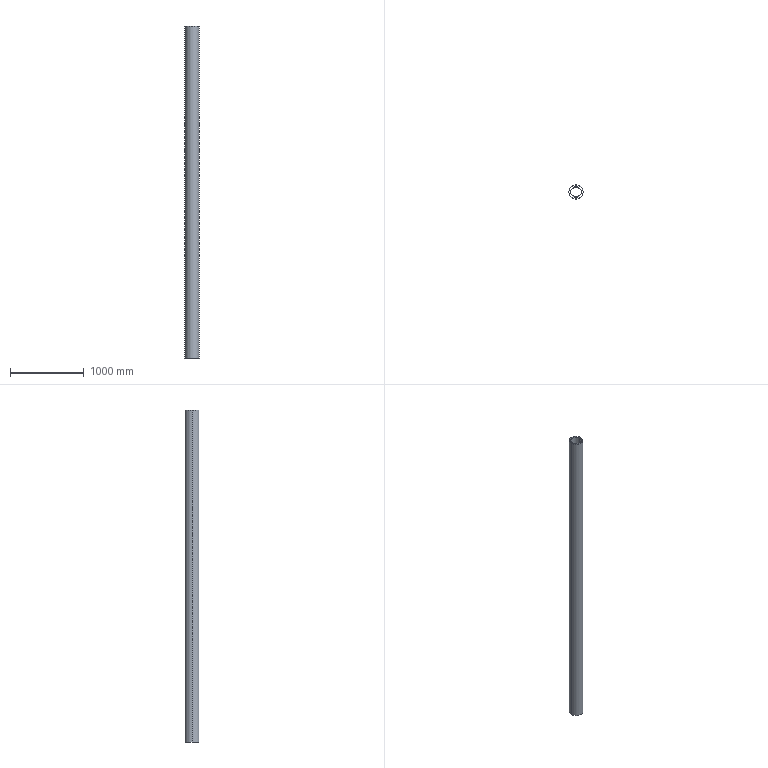Part | SolidWorks | features Extrusion 1, ICE 1 | 2 solids | 12 faces | box 190 x 190 x 4500 mm | volume 116967 mm3 | cylinder 8 | plane 4 | commonest cylinder face diameters 140.95 x2 141 x2 189.95 x2 190 x2
STEP:
#1=CARTESIAN_POINT('',(-94.975,0.,4500.));
#2=VERTEX_POINT('',#1);
#3=CARTESIAN_POINT('',(94.975,0.,4500.));
#4=VERTEX_POINT('',#3);
#5=CARTESIAN_POINT('',(0.,0.,4500.));
#6=DIRECTION('',(0.,0.,1.));
#7=DIRECTION('',(1.,0.,0.));
#8=AXIS2_PLACEMENT_3D('',#5,#6,#7);
#9=CIRCLE('',#8,94.975);
#10=EDGE_CURVE('',#2,#4,#9,.T.);
#11=ORIENTED_EDGE('',*,*,#10,.T.);
#12=CARTESIAN_POINT('',(94.975,0.,0.));
#13=VERTEX_POINT('',#12);
#14=CARTESIAN_POINT('',(94.975,0.,4500.));
#15=DIRECTION('',(0.,0.,-1.));
#16=VECTOR('',#15,1000.);
#17=LINE('',#14,#16);
#18=EDGE_CURVE('',#4,#13,#17,.T.);
#19=ORIENTED_EDGE('',*,*,#18,.T.);
#20=CARTESIAN_POINT('',(-94.975,0.,0.));
#21=VERTEX_POINT('',#20);
#22=CARTESIAN_POINT('',(0.,0.,0.));
#23=DIRECTION('',(0.,0.,1.));
#24=DIRECTION('',(1.,0.,0.));
#25=AXIS2_PLACEMENT_3D('',#22,#23,#24);
#26=CIRCLE('',#25,94.975);
#27=EDGE_CURVE('',#21,#13,#26,.T.);
#28=ORIENTED_EDGE('',*,*,#27,.F.);
#29=CARTESIAN_POINT('',(-94.975,0.,4500.));
#30=DIRECTION('',(0.,0.,-1.));
#31=VECTOR('',#30,1000.);
#32=LINE('',#29,#31);
#33=EDGE_CURVE('',#2,#21,#32,.T.);
#34=ORIENTED_EDGE('',*,*,#33,.F.);
#35=EDGE_LOOP('',(#11,#19,#28,#34));
#36=FACE_OUTER_BOUND('',#35,.T.);
#37=CARTESIAN_POINT('',(0.,0.,4500.));
#38=DIRECTION('',(0.,0.,-1.));
#39=DIRECTION('',(-1.,0.,0.));
#40=AXIS2_PLACEMENT_3D('',#37,#38,#39);
#41=CYLINDRICAL_SURFACE('',#40,94.975);
#42=ADVANCED_FACE('',(#36),#41,.F.);
#43=CARTESIAN_POINT('',(95.,0.,4500.));
#44=VERTEX_POINT('',#43);
#45=CARTESIAN_POINT('',(-95.,0.,4500.));
#46=VERTEX_POINT('',#45);
#47=CARTESIAN_POINT('',(0.,0.,4500.));
#48=DIRECTION('',(0.,0.,1.));
#49=DIRECTION('',(1.,0.,0.));
#50=AXIS2_PLACEMENT_3D('',#47,#48,#49);
#51=CIRCLE('',#50,95.);
#52=EDGE_CURVE('',#44,#46,#51,.T.);
#53=ORIENTED_EDGE('',*,*,#52,.F.);
#54=CARTESIAN_POINT('',(95.,0.,0.));
#55=VERTEX_POINT('',#54);
#56=CARTESIAN_POINT('',(95.,0.,4500.));
#57=DIRECTION('',(0.,0.,-1.));
#58=VECTOR('',#57,1000.);
#59=LINE('',#56,#58);
#60=EDGE_CURVE('',#44,#55,#59,.T.);
#61=ORIENTED_EDGE('',*,*,#60,.T.);
#62=CARTESIAN_POINT('',(-95.,0.,0.));
#63=VERTEX_POINT('',#62);
#64=CARTESIAN_POINT('',(0.,0.,0.));
#65=DIRECTION('',(0.,0.,1.));
#66=DIRECTION('',(1.,0.,0.));
#67=AXIS2_PLACEMENT_3D('',#64,#65,#66);
#68=CIRCLE('',#67,95.);
#69=EDGE_CURVE('',#55,#63,#68,.T.);
#70=ORIENTED_EDGE('',*,*,#69,.T.);
#71=CARTESIAN_POINT('',(-95.,0.,4500.));
#72=DIRECTION('',(0.,0.,-1.));
#73=VECTOR('',#72,1000.);
#74=LINE('',#71,#73);
#75=EDGE_CURVE('',#46,#63,#74,.T.);
#76=ORIENTED_EDGE('',*,*,#75,.F.);
#77=EDGE_LOOP('',(#53,#61,#70,#76));
#78=FACE_OUTER_BOUND('',#77,.T.);
#79=CARTESIAN_POINT('',(0.,0.,4500.));
#80=DIRECTION('',(0.,0.,-1.));
#81=DIRECTION('',(-1.,0.,0.));
#82=AXIS2_PLACEMENT_3D('',#79,#80,#81);
#83=CYLINDRICAL_SURFACE('',#82,95.);
#84=ADVANCED_FACE('',(#78),#83,.T.);
#85=CARTESIAN_POINT('',(0.,0.,4500.));
#86=DIRECTION('',(0.,0.,1.));
#87=DIRECTION('',(1.,0.,0.));
#88=AXIS2_PLACEMENT_3D('',#85,#86,#87);
#89=CIRCLE('',#88,95.);
#90=EDGE_CURVE('',#46,#44,#89,.T.);
#91=ORIENTED_EDGE('',*,*,#90,.T.);
#92=ORIENTED_EDGE('',*,*,#52,.T.);
#93=EDGE_LOOP('',(#91,#92));
#94=FACE_OUTER_BOUND('',#93,.T.);
#95=ORIENTED_EDGE('',*,*,#10,.F.);
#96=CARTESIAN_POINT('',(0.,0.,4500.));
#97=DIRECTION('',(0.,0.,1.));
#98=DIRECTION('',(1.,0.,0.));
#99=AXIS2_PLACEMENT_3D('',#96,#97,#98);
#100=CIRCLE('',#99,94.975);
#101=EDGE_CURVE('',#4,#2,#100,.T.);
#102=ORIENTED_EDGE('',*,*,#101,.F.);
#103=EDGE_LOOP('',(#95,#102));
#104=FACE_BOUND('',#103,.T.);
#105=CARTESIAN_POINT('',(0.,0.,4500.));
#106=DIRECTION('',(0.,0.,1.));
#107=DIRECTION('',(1.,0.,0.));
#108=AXIS2_PLACEMENT_3D('',#105,#106,#107);
#109=PLANE('',#108);
#110=ADVANCED_FACE('',(#94,#104),#109,.T.);
#111=CARTESIAN_POINT('',(0.,0.,0.));
#112=DIRECTION('',(0.,0.,1.));
#113=DIRECTION('',(1.,0.,0.));
#114=AXIS2_PLACEMENT_3D('',#111,#112,#113);
#115=CIRCLE('',#114,95.);
#116=EDGE_CURVE('',#63,#55,#115,.T.);
#117=ORIENTED_EDGE('',*,*,#116,.F.);
#118=ORIENTED_EDGE('',*,*,#69,.F.);
#119=EDGE_LOOP('',(#117,#118));
#120=FACE_OUTER_BOUND('',#119,.T.);
#121=ORIENTED_EDGE('',*,*,#27,.T.);
#122=CARTESIAN_POINT('',(0.,0.,0.));
#123=DIRECTION('',(0.,0.,1.));
#124=DIRECTION('',(1.,0.,0.));
#125=AXIS2_PLACEMENT_3D('',#122,#123,#124);
#126=CIRCLE('',#125,94.975);
#127=EDGE_CURVE('',#13,#21,#126,.T.);
#128=ORIENTED_EDGE('',*,*,#127,.T.);
#129=EDGE_LOOP('',(#121,#128));
#130=FACE_BOUND('',#129,.T.);
#131=CARTESIAN_POINT('',(0.,0.,0.));
#132=DIRECTION('',(0.,0.,1.));
#133=DIRECTION('',(1.,0.,0.));
#134=AXIS2_PLACEMENT_3D('',#131,#132,#133);
#135=PLANE('',#134);
#136=ADVANCED_FACE('',(#120,#130),#135,.F.);
#137=ORIENTED_EDGE('',*,*,#60,.F.);
#138=ORIENTED_EDGE('',*,*,#90,.F.);
#139=ORIENTED_EDGE('',*,*,#75,.T.);
#140=ORIENTED_EDGE('',*,*,#116,.T.);
#141=EDGE_LOOP('',(#137,#138,#139,#140));
#142=FACE_OUTER_BOUND('',#141,.T.);
#143=CARTESIAN_POINT('',(0.,0.,4500.));
#144=DIRECTION('',(0.,0.,-1.));
#145=DIRECTION('',(-1.,0.,0.));
#146=AXIS2_PLACEMENT_3D('',#143,#144,#145);
#147=CYLINDRICAL_SURFACE('',#146,95.);
#148=ADVANCED_FACE('',(#142),#147,.T.);
#149=ORIENTED_EDGE('',*,*,#18,.F.);
#150=ORIENTED_EDGE('',*,*,#101,.T.);
#151=ORIENTED_EDGE('',*,*,#33,.T.);
#152=ORIENTED_EDGE('',*,*,#127,.F.);
#153=EDGE_LOOP('',(#149,#150,#151,#152));
#154=FACE_OUTER_BOUND('',#153,.T.);
#155=CARTESIAN_POINT('',(0.,0.,4500.));
#156=DIRECTION('',(0.,0.,-1.));
#157=DIRECTION('',(-1.,0.,0.));
#158=AXIS2_PLACEMENT_3D('',#155,#156,#157);
#159=CYLINDRICAL_SURFACE('',#158,94.975);
#160=ADVANCED_FACE('',(#154),#159,.F.);
#161=CLOSED_SHELL('',(#42,#84,#110,#136,#148,#160));
#162=MANIFOLD_SOLID_BREP('',#161);
#163=CARTESIAN_POINT('',(-70.475,0.,4500.));
#164=VERTEX_POINT('',#163);
#165=CARTESIAN_POINT('',(70.475,0.,4500.));
#166=VERTEX_POINT('',#165);
#167=CARTESIAN_POINT('',(0.,0.,4500.));
#168=DIRECTION('',(0.,0.,1.));
#169=DIRECTION('',(1.,0.,0.));
#170=AXIS2_PLACEMENT_3D('',#167,#168,#169);
#171=CIRCLE('',#170,70.475);
#172=EDGE_CURVE('',#164,#166,#171,.T.);
#173=ORIENTED_EDGE('',*,*,#172,.T.);
#174=CARTESIAN_POINT('',(70.475,0.,0.));
#175=VERTEX_POINT('',#174);
#176=CARTESIAN_POINT('',(70.475,0.,4500.));
#177=DIRECTION('',(0.,0.,-1.));
#178=VECTOR('',#177,1000.);
#179=LINE('',#176,#178);
#180=EDGE_CURVE('',#166,#175,#179,.T.);
#181=ORIENTED_EDGE('',*,*,#180,.T.);
#182=CARTESIAN_POINT('',(-70.475,0.,0.));
#183=VERTEX_POINT('',#182);
#184=CARTESIAN_POINT('',(0.,0.,0.));
#185=DIRECTION('',(0.,0.,1.));
#186=DIRECTION('',(1.,0.,0.));
#187=AXIS2_PLACEMENT_3D('',#184,#185,#186);
#188=CIRCLE('',#187,70.475);
#189=EDGE_CURVE('',#183,#175,#188,.T.);
#190=ORIENTED_EDGE('',*,*,#189,.F.);
#191=CARTESIAN_POINT('',(-70.475,0.,4500.));
#192=DIRECTION('',(0.,0.,-1.));
#193=VECTOR('',#192,1000.);
#194=LINE('',#191,#193);
#195=EDGE_CURVE('',#164,#183,#194,.T.);
#196=ORIENTED_EDGE('',*,*,#195,.F.);
#197=EDGE_LOOP('',(#173,#181,#190,#196));
#198=FACE_OUTER_BOUND('',#197,.T.);
#199=CARTESIAN_POINT('',(0.,0.,4500.));
#200=DIRECTION('',(0.,0.,-1.));
#201=DIRECTION('',(-1.,0.,0.));
#202=AXIS2_PLACEMENT_3D('',#199,#200,#201);
#203=CYLINDRICAL_SURFACE('',#202,70.475);
#204=ADVANCED_FACE('',(#198),#203,.F.);
#205=CARTESIAN_POINT('',(70.5,0.,4500.));
#206=VERTEX_POINT('',#205);
#207=CARTESIAN_POINT('',(-70.5,0.,4500.));
#208=VERTEX_POINT('',#207);
#209=CARTESIAN_POINT('',(0.,0.,4500.));
#210=DIRECTION('',(0.,0.,1.));
#211=DIRECTION('',(1.,0.,0.));
#212=AXIS2_PLACEMENT_3D('',#209,#210,#211);
#213=CIRCLE('',#212,70.5);
#214=EDGE_CURVE('',#206,#208,#213,.T.);
#215=ORIENTED_EDGE('',*,*,#214,.F.);
#216=CARTESIAN_POINT('',(70.5,0.,0.));
#217=VERTEX_POINT('',#216);
#218=CARTESIAN_POINT('',(70.5,0.,4500.));
#219=DIRECTION('',(0.,0.,-1.));
#220=VECTOR('',#219,1000.);
#221=LINE('',#218,#220);
#222=EDGE_CURVE('',#206,#217,#221,.T.);
#223=ORIENTED_EDGE('',*,*,#222,.T.);
#224=CARTESIAN_POINT('',(-70.5,0.,0.));
#225=VERTEX_POINT('',#224);
#226=CARTESIAN_POINT('',(0.,0.,0.));
#227=DIRECTION('',(0.,0.,1.));
#228=DIRECTION('',(1.,0.,0.));
#229=AXIS2_PLACEMENT_3D('',#226,#227,#228);
#230=CIRCLE('',#229,70.5);
#231=EDGE_CURVE('',#217,#225,#230,.T.);
#232=ORIENTED_EDGE('',*,*,#231,.T.);
#233=CARTESIAN_POINT('',(-70.5,0.,4500.));
#234=DIRECTION('',(0.,0.,-1.));
#235=VECTOR('',#234,1000.);
#236=LINE('',#233,#235);
#237=EDGE_CURVE('',#208,#225,#236,.T.);
#238=ORIENTED_EDGE('',*,*,#237,.F.);
#239=EDGE_LOOP('',(#215,#223,#232,#238));
#240=FACE_OUTER_BOUND('',#239,.T.);
#241=CARTESIAN_POINT('',(0.,0.,4500.));
#242=DIRECTION('',(0.,0.,-1.));
#243=DIRECTION('',(-1.,0.,0.));
#244=AXIS2_PLACEMENT_3D('',#241,#242,#243);
#245=CYLINDRICAL_SURFACE('',#244,70.5);
#246=ADVANCED_FACE('',(#240),#245,.T.);
#247=CARTESIAN_POINT('',(0.,0.,4500.));
#248=DIRECTION('',(0.,0.,1.));
#249=DIRECTION('',(1.,0.,0.));
#250=AXIS2_PLACEMENT_3D('',#247,#248,#249);
#251=CIRCLE('',#250,70.5);
#252=EDGE_CURVE('',#208,#206,#251,.T.);
#253=ORIENTED_EDGE('',*,*,#252,.T.);
#254=ORIENTED_EDGE('',*,*,#214,.T.);
#255=EDGE_LOOP('',(#253,#254));
#256=FACE_OUTER_BOUND('',#255,.T.);
#257=ORIENTED_EDGE('',*,*,#172,.F.);
#258=CARTESIAN_POINT('',(0.,0.,4500.));
#259=DIRECTION('',(0.,0.,1.));
#260=DIRECTION('',(1.,0.,0.));
#261=AXIS2_PLACEMENT_3D('',#258,#259,#260);
#262=CIRCLE('',#261,70.475);
#263=EDGE_CURVE('',#166,#164,#262,.T.);
#264=ORIENTED_EDGE('',*,*,#263,.F.);
#265=EDGE_LOOP('',(#257,#264));
#266=FACE_BOUND('',#265,.T.);
#267=CARTESIAN_POINT('',(0.,0.,4500.));
#268=DIRECTION('',(0.,0.,1.));
#269=DIRECTION('',(1.,0.,0.));
#270=AXIS2_PLACEMENT_3D('',#267,#268,#269);
#271=PLANE('',#270);
#272=ADVANCED_FACE('',(#256,#266),#271,.T.);
#273=CARTESIAN_POINT('',(0.,0.,0.));
#274=DIRECTION('',(0.,0.,1.));
#275=DIRECTION('',(1.,0.,0.));
#276=AXIS2_PLACEMENT_3D('',#273,#274,#275);
#277=CIRCLE('',#276,70.5);
#278=EDGE_CURVE('',#225,#217,#277,.T.);
#279=ORIENTED_EDGE('',*,*,#278,.F.);
#280=ORIENTED_EDGE('',*,*,#231,.F.);
#281=EDGE_LOOP('',(#279,#280));
#282=FACE_OUTER_BOUND('',#281,.T.);
#283=ORIENTED_EDGE('',*,*,#189,.T.);
#284=CARTESIAN_POINT('',(0.,0.,0.));
#285=DIRECTION('',(0.,0.,1.));
#286=DIRECTION('',(1.,0.,0.));
#287=AXIS2_PLACEMENT_3D('',#284,#285,#286);
#288=CIRCLE('',#287,70.475);
#289=EDGE_CURVE('',#175,#183,#288,.T.);
#290=ORIENTED_EDGE('',*,*,#289,.T.);
#291=EDGE_LOOP('',(#283,#290));
#292=FACE_BOUND('',#291,.T.);
#293=CARTESIAN_POINT('',(0.,0.,0.));
#294=DIRECTION('',(0.,0.,1.));
#295=DIRECTION('',(1.,0.,0.));
#296=AXIS2_PLACEMENT_3D('',#293,#294,#295);
#297=PLANE('',#296);
#298=ADVANCED_FACE('',(#282,#292),#297,.F.);
#299=ORIENTED_EDGE('',*,*,#222,.F.);
#300=ORIENTED_EDGE('',*,*,#252,.F.);
#301=ORIENTED_EDGE('',*,*,#237,.T.);
#302=ORIENTED_EDGE('',*,*,#278,.T.);
#303=EDGE_LOOP('',(#299,#300,#301,#302));
#304=FACE_OUTER_BOUND('',#303,.T.);
#305=CARTESIAN_POINT('',(0.,0.,4500.));
#306=DIRECTION('',(0.,0.,-1.));
#307=DIRECTION('',(-1.,0.,0.));
#308=AXIS2_PLACEMENT_3D('',#305,#306,#307);
#309=CYLINDRICAL_SURFACE('',#308,70.5);
#310=ADVANCED_FACE('',(#304),#309,.T.);
#311=ORIENTED_EDGE('',*,*,#180,.F.);
#312=ORIENTED_EDGE('',*,*,#263,.T.);
#313=ORIENTED_EDGE('',*,*,#195,.T.);
#314=ORIENTED_EDGE('',*,*,#289,.F.);
#315=EDGE_LOOP('',(#311,#312,#313,#314));
#316=FACE_OUTER_BOUND('',#315,.T.);
#317=CARTESIAN_POINT('',(0.,0.,4500.));
#318=DIRECTION('',(0.,0.,-1.));
#319=DIRECTION('',(-1.,0.,0.));
#320=AXIS2_PLACEMENT_3D('',#317,#318,#319);
#321=CYLINDRICAL_SURFACE('',#320,70.475);
#322=ADVANCED_FACE('',(#316),#321,.F.);
#323=CLOSED_SHELL('',(#204,#246,#272,#298,#310,#322));
#324=MANIFOLD_SOLID_BREP('',#323);
#325=CARTESIAN_POINT('',(0.,0.,0.));
#326=DIRECTION('',(0.,0.,1.));
#327=DIRECTION('',(1.,0.,0.));
#328=AXIS2_PLACEMENT_3D('',#325,#326,#327);
#329=(LENGTH_UNIT()NAMED_UNIT(*)SI_UNIT(.MILLI.,.METRE.));
#330=UNCERTAINTY_MEASURE_WITH_UNIT(LENGTH_MEASURE(0.00001),#329,'','');
#331=(NAMED_UNIT(*)PLANE_ANGLE_UNIT()SI_UNIT($,.RADIAN.));
#332=(NAMED_UNIT(*)SI_UNIT($,.STERADIAN.)SOLID_ANGLE_UNIT());
#333=(GEOMETRIC_REPRESENTATION_CONTEXT(3)GLOBAL_UNCERTAINTY_ASSIGNED_CONTEXT((#330))GLOBAL_UNIT_ASSIGNED_CONTEXT((#329,#331,#332))REPRESENTATION_CONTEXT('',''));
#334=ADVANCED_BREP_SHAPE_REPRESENTATION('',(#162,#324,#328),#333);